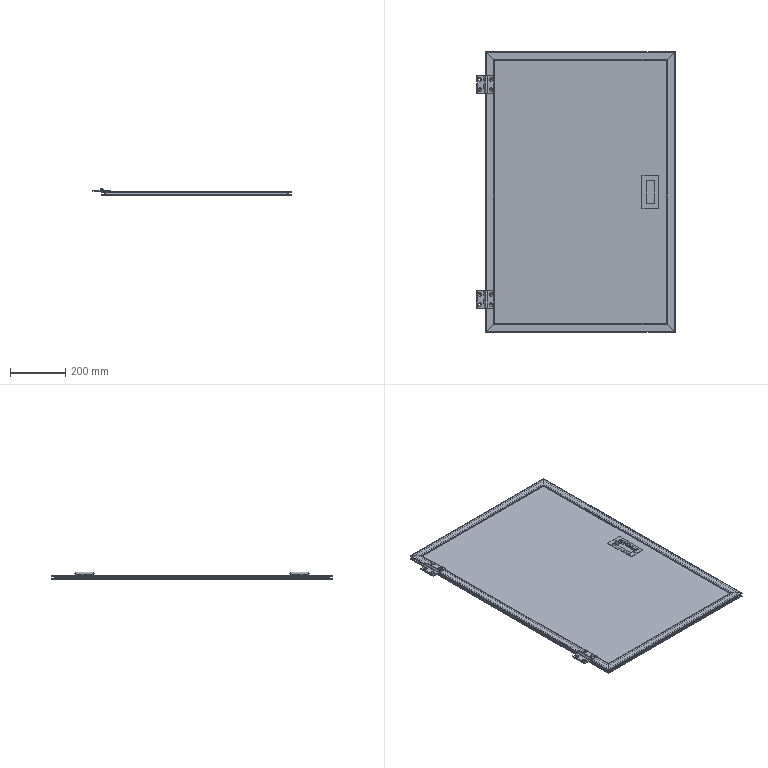Part | SolidWorks | features MoveCopyBody 3, Stock 3, ICE 2, HoleWzd 1, WeldMemberFeat 1, WeldmentFeature 1 | 8 solids | 319 faces | box 718 x 1016 x 28.7 mm | volume 4599989 mm3 | plane 165 | cylinder 110 | cone 36 | sphere 8 | commonest cylinder face diameters 5 x28 2 x20 10 x16 4 x12 15 x10 6.4 x8